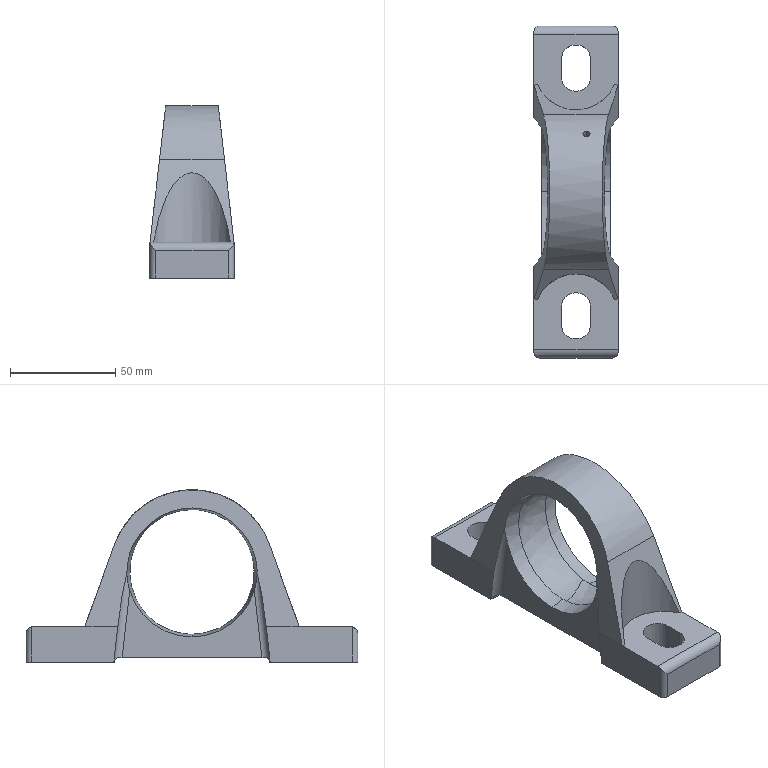Part | SolidWorks | features BaseBody 1 | 1 solid | 49 faces | box 40 x 158 x 82 mm | volume 137607 mm3 | plane 22 | cylinder 21 | cone 4 | spline 2 | commonest cylinder face diameters 5.333 x4 7.5 x4 14 x4 3.5 x2 4 x2 8 x2